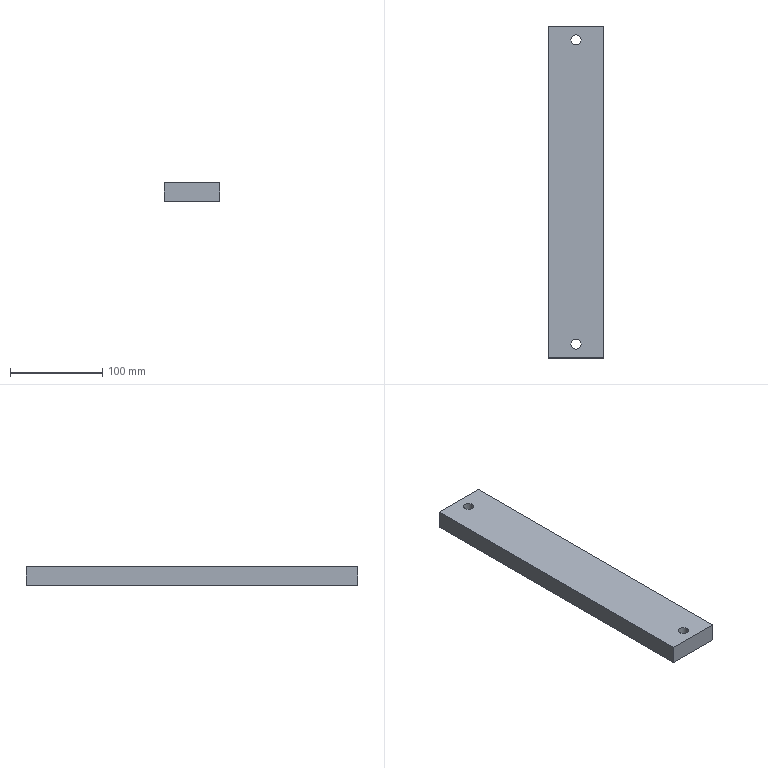Part | STEP file | 1 solid | 12 faces | box 60 x 360 x 20 mm | volume 425296 mm3 | plane 8 | cylinder 4 | commonest cylinder face diameters 11 x2 17 x2
STEP:
#1=CARTESIAN_POINT('',(0.,0.,0.));
#2=DIRECTION('',(0.,0.,1.));
#3=DIRECTION('',(1.,0.,0.));
#4=AXIS2_PLACEMENT_3D('',#1,#2,#3);
#5=CARTESIAN_POINT('',(1452.247,622.48,-145.381));
#6=VERTEX_POINT('',#5);
#7=CARTESIAN_POINT('',(1512.247,622.48,-145.381));
#8=VERTEX_POINT('',#7);
#9=CARTESIAN_POINT('',(1452.247,622.48,-145.381));
#10=DIRECTION('',(1.,0.,0.));
#11=VECTOR('',#10,1.);
#12=LINE('',#9,#11);
#13=CARTESIAN_POINT('',(1452.247,622.48,-165.381));
#14=DIRECTION('',(0.,-1.,0.));
#15=DIRECTION('',(0.,0.,1.));
#16=AXIS2_PLACEMENT_3D('',#13,#14,#15);
#17=PLANE('',#16);
#18=CARTESIAN_POINT('',(20.,0.));
#19=DIRECTION('',(0.,-1.));
#20=VECTOR('',#19,1.);
#21=LINE('',#18,#20);
#22=(GEOMETRIC_REPRESENTATION_CONTEXT(2)PARAMETRIC_REPRESENTATION_CONTEXT()REPRESENTATION_CONTEXT('',''));
#23=DEFINITIONAL_REPRESENTATION('',(#21),#22);
#24=PCURVE('',#17,#23);
#25=CARTESIAN_POINT('',(-340.,0.,-145.381));
#26=DIRECTION('',(0.,0.,-1.));
#27=DIRECTION('',(1.,0.,0.));
#28=AXIS2_PLACEMENT_3D('',#25,#26,#27);
#29=PLANE('',#28);
#30=CARTESIAN_POINT('',(1792.247,-622.48));
#31=DIRECTION('',(1.,0.));
#32=VECTOR('',#31,1.);
#33=LINE('',#30,#32);
#34=(GEOMETRIC_REPRESENTATION_CONTEXT(2)PARAMETRIC_REPRESENTATION_CONTEXT()REPRESENTATION_CONTEXT('',''));
#35=DEFINITIONAL_REPRESENTATION('',(#33),#34);
#36=PCURVE('',#29,#35);
#37=SURFACE_CURVE('',#12,(#24,#36),.PCURVE_S1.);
#38=EDGE_CURVE('',#6,#8,#37,.T.);
#39=ORIENTED_EDGE('',*,*,#38,.T.);
#40=CARTESIAN_POINT('',(1512.247,622.48,-165.381));
#41=VERTEX_POINT('',#40);
#42=CARTESIAN_POINT('',(1512.247,622.48,-165.381));
#43=DIRECTION('',(0.,0.,1.));
#44=VECTOR('',#43,1.);
#45=LINE('',#42,#44);
#46=CARTESIAN_POINT('',(0.,-60.));
#47=DIRECTION('',(1.,0.));
#48=VECTOR('',#47,1.);
#49=LINE('',#46,#48);
#50=(GEOMETRIC_REPRESENTATION_CONTEXT(2)PARAMETRIC_REPRESENTATION_CONTEXT()REPRESENTATION_CONTEXT('',''));
#51=DEFINITIONAL_REPRESENTATION('',(#49),#50);
#52=PCURVE('',#17,#51);
#53=CARTESIAN_POINT('',(1512.247,632.48,-165.381));
#54=DIRECTION('',(-1.,0.,0.));
#55=DIRECTION('',(0.,0.,-1.));
#56=AXIS2_PLACEMENT_3D('',#53,#54,#55);
#57=PLANE('',#56);
#58=CARTESIAN_POINT('',(0.,10.));
#59=DIRECTION('',(-1.,0.));
#60=VECTOR('',#59,1.);
#61=LINE('',#58,#60);
#62=(GEOMETRIC_REPRESENTATION_CONTEXT(2)PARAMETRIC_REPRESENTATION_CONTEXT()REPRESENTATION_CONTEXT('',''));
#63=DEFINITIONAL_REPRESENTATION('',(#61),#62);
#64=PCURVE('',#57,#63);
#65=SURFACE_CURVE('',#45,(#52,#64),.PCURVE_S1.);
#66=EDGE_CURVE('',#41,#8,#65,.T.);
#67=ORIENTED_EDGE('',*,*,#66,.F.);
#68=CARTESIAN_POINT('',(1452.247,622.48,-165.381));
#69=VERTEX_POINT('',#68);
#70=CARTESIAN_POINT('',(1452.247,622.48,-165.381));
#71=DIRECTION('',(1.,0.,0.));
#72=VECTOR('',#71,1.);
#73=LINE('',#70,#72);
#74=CARTESIAN_POINT('',(0.,0.));
#75=DIRECTION('',(0.,-1.));
#76=VECTOR('',#75,1.);
#77=LINE('',#74,#76);
#78=(GEOMETRIC_REPRESENTATION_CONTEXT(2)PARAMETRIC_REPRESENTATION_CONTEXT()REPRESENTATION_CONTEXT('',''));
#79=DEFINITIONAL_REPRESENTATION('',(#77),#78);
#80=PCURVE('',#17,#79);
#81=CARTESIAN_POINT('',(-340.,0.,-165.381));
#82=DIRECTION('',(0.,0.,-1.));
#83=DIRECTION('',(1.,0.,0.));
#84=AXIS2_PLACEMENT_3D('',#81,#82,#83);
#85=PLANE('',#84);
#86=CARTESIAN_POINT('',(1792.247,-622.48));
#87=DIRECTION('',(1.,0.));
#88=VECTOR('',#87,1.);
#89=LINE('',#86,#88);
#90=(GEOMETRIC_REPRESENTATION_CONTEXT(2)PARAMETRIC_REPRESENTATION_CONTEXT()REPRESENTATION_CONTEXT('',''));
#91=DEFINITIONAL_REPRESENTATION('',(#89),#90);
#92=PCURVE('',#85,#91);
#93=SURFACE_CURVE('',#73,(#80,#92),.PCURVE_S1.);
#94=EDGE_CURVE('',#69,#41,#93,.T.);
#95=ORIENTED_EDGE('',*,*,#94,.F.);
#96=CARTESIAN_POINT('',(1452.247,622.48,-165.381));
#97=DIRECTION('',(0.,0.,1.));
#98=VECTOR('',#97,1.);
#99=LINE('',#96,#98);
#100=CARTESIAN_POINT('',(0.,0.));
#101=DIRECTION('',(1.,0.));
#102=VECTOR('',#101,1.);
#103=LINE('',#100,#102);
#104=(GEOMETRIC_REPRESENTATION_CONTEXT(2)PARAMETRIC_REPRESENTATION_CONTEXT()REPRESENTATION_CONTEXT('',''));
#105=DEFINITIONAL_REPRESENTATION('',(#103),#104);
#106=PCURVE('',#17,#105);
#107=CARTESIAN_POINT('',(1452.247,252.48,-165.381));
#108=DIRECTION('',(1.,0.,0.));
#109=DIRECTION('',(0.,0.,1.));
#110=AXIS2_PLACEMENT_3D('',#107,#108,#109);
#111=PLANE('',#110);
#112=CARTESIAN_POINT('',(0.,-370.));
#113=DIRECTION('',(1.,0.));
#114=VECTOR('',#113,1.);
#115=LINE('',#112,#114);
#116=(GEOMETRIC_REPRESENTATION_CONTEXT(2)PARAMETRIC_REPRESENTATION_CONTEXT()REPRESENTATION_CONTEXT('',''));
#117=DEFINITIONAL_REPRESENTATION('',(#115),#116);
#118=PCURVE('',#111,#117);
#119=SURFACE_CURVE('',#99,(#106,#118),.PCURVE_S1.);
#120=EDGE_CURVE('',#69,#6,#119,.T.);
#121=ORIENTED_EDGE('',*,*,#120,.T.);
#122=EDGE_LOOP('',(#39,#67,#95,#121));
#123=FACE_BOUND('',#122,.T.);
#124=ADVANCED_FACE('',(#123),#17,.F.);
#125=CARTESIAN_POINT('',(1512.247,262.48,-145.381));
#126=VERTEX_POINT('',#125);
#127=CARTESIAN_POINT('',(1512.247,632.48,-145.381));
#128=DIRECTION('',(0.,-1.,0.));
#129=VECTOR('',#128,1.);
#130=LINE('',#127,#129);
#131=CARTESIAN_POINT('',(-20.,0.));
#132=DIRECTION('',(0.,1.));
#133=VECTOR('',#132,1.);
#134=LINE('',#131,#133);
#135=(GEOMETRIC_REPRESENTATION_CONTEXT(2)PARAMETRIC_REPRESENTATION_CONTEXT()REPRESENTATION_CONTEXT('',''));
#136=DEFINITIONAL_REPRESENTATION('',(#134),#135);
#137=PCURVE('',#57,#136);
#138=CARTESIAN_POINT('',(1852.247,-632.48));
#139=DIRECTION('',(0.,1.));
#140=VECTOR('',#139,1.);
#141=LINE('',#138,#140);
#142=(GEOMETRIC_REPRESENTATION_CONTEXT(2)PARAMETRIC_REPRESENTATION_CONTEXT()REPRESENTATION_CONTEXT('',''));
#143=DEFINITIONAL_REPRESENTATION('',(#141),#142);
#144=PCURVE('',#29,#143);
#145=SURFACE_CURVE('',#130,(#137,#144),.PCURVE_S1.);
#146=EDGE_CURVE('',#8,#126,#145,.T.);
#147=ORIENTED_EDGE('',*,*,#146,.T.);
#148=CARTESIAN_POINT('',(1512.247,262.48,-165.381));
#149=VERTEX_POINT('',#148);
#150=CARTESIAN_POINT('',(1512.247,262.48,-165.381));
#151=DIRECTION('',(0.,0.,1.));
#152=VECTOR('',#151,1.);
#153=LINE('',#150,#152);
#154=CARTESIAN_POINT('',(0.,370.));
#155=DIRECTION('',(-1.,0.));
#156=VECTOR('',#155,1.);
#157=LINE('',#154,#156);
#158=(GEOMETRIC_REPRESENTATION_CONTEXT(2)PARAMETRIC_REPRESENTATION_CONTEXT()REPRESENTATION_CONTEXT('',''));
#159=DEFINITIONAL_REPRESENTATION('',(#157),#158);
#160=PCURVE('',#57,#159);
#161=CARTESIAN_POINT('',(1512.247,262.48,-165.381));
#162=DIRECTION('',(0.,1.,0.));
#163=DIRECTION('',(1.,0.,0.));
#164=AXIS2_PLACEMENT_3D('',#161,#162,#163);
#165=PLANE('',#164);
#166=CARTESIAN_POINT('',(0.,0.));
#167=DIRECTION('',(0.,-1.));
#168=VECTOR('',#167,1.);
#169=LINE('',#166,#168);
#170=(GEOMETRIC_REPRESENTATION_CONTEXT(2)PARAMETRIC_REPRESENTATION_CONTEXT()REPRESENTATION_CONTEXT('',''));
#171=DEFINITIONAL_REPRESENTATION('',(#169),#170);
#172=PCURVE('',#165,#171);
#173=SURFACE_CURVE('',#153,(#160,#172),.PCURVE_S1.);
#174=EDGE_CURVE('',#149,#126,#173,.T.);
#175=ORIENTED_EDGE('',*,*,#174,.F.);
#176=CARTESIAN_POINT('',(1512.247,632.48,-165.381));
#177=DIRECTION('',(0.,-1.,0.));
#178=VECTOR('',#177,1.);
#179=LINE('',#176,#178);
#180=CARTESIAN_POINT('',(0.,0.));
#181=DIRECTION('',(0.,1.));
#182=VECTOR('',#181,1.);
#183=LINE('',#180,#182);
#184=(GEOMETRIC_REPRESENTATION_CONTEXT(2)PARAMETRIC_REPRESENTATION_CONTEXT()REPRESENTATION_CONTEXT('',''));
#185=DEFINITIONAL_REPRESENTATION('',(#183),#184);
#186=PCURVE('',#57,#185);
#187=CARTESIAN_POINT('',(1852.247,-632.48));
#188=DIRECTION('',(0.,1.));
#189=VECTOR('',#188,1.);
#190=LINE('',#187,#189);
#191=(GEOMETRIC_REPRESENTATION_CONTEXT(2)PARAMETRIC_REPRESENTATION_CONTEXT()REPRESENTATION_CONTEXT('',''));
#192=DEFINITIONAL_REPRESENTATION('',(#190),#191);
#193=PCURVE('',#85,#192);
#194=SURFACE_CURVE('',#179,(#186,#193),.PCURVE_S1.);
#195=EDGE_CURVE('',#41,#149,#194,.T.);
#196=ORIENTED_EDGE('',*,*,#195,.F.);
#197=ORIENTED_EDGE('',*,*,#66,.T.);
#198=EDGE_LOOP('',(#147,#175,#196,#197));
#199=FACE_BOUND('',#198,.T.);
#200=ADVANCED_FACE('',(#199),#57,.F.);
#201=CARTESIAN_POINT('',(1452.247,262.48,-145.381));
#202=VERTEX_POINT('',#201);
#203=CARTESIAN_POINT('',(1512.247,262.48,-145.381));
#204=DIRECTION('',(-1.,0.,0.));
#205=VECTOR('',#204,1.);
#206=LINE('',#203,#205);
#207=CARTESIAN_POINT('',(0.,-20.));
#208=DIRECTION('',(-1.,0.));
#209=VECTOR('',#208,1.);
#210=LINE('',#207,#209);
#211=(GEOMETRIC_REPRESENTATION_CONTEXT(2)PARAMETRIC_REPRESENTATION_CONTEXT()REPRESENTATION_CONTEXT('',''));
#212=DEFINITIONAL_REPRESENTATION('',(#210),#211);
#213=PCURVE('',#165,#212);
#214=CARTESIAN_POINT('',(1852.247,-262.48));
#215=DIRECTION('',(-1.,0.));
#216=VECTOR('',#215,1.);
#217=LINE('',#214,#216);
#218=(GEOMETRIC_REPRESENTATION_CONTEXT(2)PARAMETRIC_REPRESENTATION_CONTEXT()REPRESENTATION_CONTEXT('',''));
#219=DEFINITIONAL_REPRESENTATION('',(#217),#218);
#220=PCURVE('',#29,#219);
#221=SURFACE_CURVE('',#206,(#213,#220),.PCURVE_S1.);
#222=EDGE_CURVE('',#126,#202,#221,.T.);
#223=ORIENTED_EDGE('',*,*,#222,.T.);
#224=CARTESIAN_POINT('',(1452.247,262.48,-165.381));
#225=VERTEX_POINT('',#224);
#226=CARTESIAN_POINT('',(1452.247,262.48,-165.381));
#227=DIRECTION('',(0.,0.,1.));
#228=VECTOR('',#227,1.);
#229=LINE('',#226,#228);
#230=CARTESIAN_POINT('',(-60.,0.));
#231=DIRECTION('',(0.,-1.));
#232=VECTOR('',#231,1.);
#233=LINE('',#230,#232);
#234=(GEOMETRIC_REPRESENTATION_CONTEXT(2)PARAMETRIC_REPRESENTATION_CONTEXT()REPRESENTATION_CONTEXT('',''));
#235=DEFINITIONAL_REPRESENTATION('',(#233),#234);
#236=PCURVE('',#165,#235);
#237=CARTESIAN_POINT('',(0.,-10.));
#238=DIRECTION('',(1.,0.));
#239=VECTOR('',#238,1.);
#240=LINE('',#237,#239);
#241=(GEOMETRIC_REPRESENTATION_CONTEXT(2)PARAMETRIC_REPRESENTATION_CONTEXT()REPRESENTATION_CONTEXT('',''));
#242=DEFINITIONAL_REPRESENTATION('',(#240),#241);
#243=PCURVE('',#111,#242);
#244=SURFACE_CURVE('',#229,(#236,#243),.PCURVE_S1.);
#245=EDGE_CURVE('',#225,#202,#244,.T.);
#246=ORIENTED_EDGE('',*,*,#245,.F.);
#247=CARTESIAN_POINT('',(1512.247,262.48,-165.381));
#248=DIRECTION('',(-1.,0.,0.));
#249=VECTOR('',#248,1.);
#250=LINE('',#247,#249);
#251=CARTESIAN_POINT('',(0.,0.));
#252=DIRECTION('',(-1.,0.));
#253=VECTOR('',#252,1.);
#254=LINE('',#251,#253);
#255=(GEOMETRIC_REPRESENTATION_CONTEXT(2)PARAMETRIC_REPRESENTATION_CONTEXT()REPRESENTATION_CONTEXT('',''));
#256=DEFINITIONAL_REPRESENTATION('',(#254),#255);
#257=PCURVE('',#165,#256);
#258=CARTESIAN_POINT('',(1852.247,-262.48));
#259=DIRECTION('',(-1.,0.));
#260=VECTOR('',#259,1.);
#261=LINE('',#258,#260);
#262=(GEOMETRIC_REPRESENTATION_CONTEXT(2)PARAMETRIC_REPRESENTATION_CONTEXT()REPRESENTATION_CONTEXT('',''));
#263=DEFINITIONAL_REPRESENTATION('',(#261),#262);
#264=PCURVE('',#85,#263);
#265=SURFACE_CURVE('',#250,(#257,#264),.PCURVE_S1.);
#266=EDGE_CURVE('',#149,#225,#265,.T.);
#267=ORIENTED_EDGE('',*,*,#266,.F.);
#268=ORIENTED_EDGE('',*,*,#174,.T.);
#269=EDGE_LOOP('',(#223,#246,#267,#268));
#270=FACE_BOUND('',#269,.T.);
#271=ADVANCED_FACE('',(#270),#165,.F.);
#272=CARTESIAN_POINT('',(1452.247,252.48,-145.381));
#273=DIRECTION('',(0.,1.,0.));
#274=VECTOR('',#273,1.);
#275=LINE('',#272,#274);
#276=CARTESIAN_POINT('',(20.,0.));
#277=DIRECTION('',(0.,-1.));
#278=VECTOR('',#277,1.);
#279=LINE('',#276,#278);
#280=(GEOMETRIC_REPRESENTATION_CONTEXT(2)PARAMETRIC_REPRESENTATION_CONTEXT()REPRESENTATION_CONTEXT('',''));
#281=DEFINITIONAL_REPRESENTATION('',(#279),#280);
#282=PCURVE('',#111,#281);
#283=CARTESIAN_POINT('',(1792.247,-252.48));
#284=DIRECTION('',(0.,-1.));
#285=VECTOR('',#284,1.);
#286=LINE('',#283,#285);
#287=(GEOMETRIC_REPRESENTATION_CONTEXT(2)PARAMETRIC_REPRESENTATION_CONTEXT()REPRESENTATION_CONTEXT('',''));
#288=DEFINITIONAL_REPRESENTATION('',(#286),#287);
#289=PCURVE('',#29,#288);
#290=SURFACE_CURVE('',#275,(#282,#289),.PCURVE_S1.);
#291=EDGE_CURVE('',#202,#6,#290,.T.);
#292=ORIENTED_EDGE('',*,*,#291,.T.);
#293=ORIENTED_EDGE('',*,*,#120,.F.);
#294=CARTESIAN_POINT('',(1452.247,252.48,-165.381));
#295=DIRECTION('',(0.,1.,0.));
#296=VECTOR('',#295,1.);
#297=LINE('',#294,#296);
#298=CARTESIAN_POINT('',(0.,0.));
#299=DIRECTION('',(0.,-1.));
#300=VECTOR('',#299,1.);
#301=LINE('',#298,#300);
#302=(GEOMETRIC_REPRESENTATION_CONTEXT(2)PARAMETRIC_REPRESENTATION_CONTEXT()REPRESENTATION_CONTEXT('',''));
#303=DEFINITIONAL_REPRESENTATION('',(#301),#302);
#304=PCURVE('',#111,#303);
#305=CARTESIAN_POINT('',(1792.247,-252.48));
#306=DIRECTION('',(0.,-1.));
#307=VECTOR('',#306,1.);
#308=LINE('',#305,#307);
#309=(GEOMETRIC_REPRESENTATION_CONTEXT(2)PARAMETRIC_REPRESENTATION_CONTEXT()REPRESENTATION_CONTEXT('',''));
#310=DEFINITIONAL_REPRESENTATION('',(#308),#309);
#311=PCURVE('',#85,#310);
#312=SURFACE_CURVE('',#297,(#304,#311),.PCURVE_S1.);
#313=EDGE_CURVE('',#225,#69,#312,.T.);
#314=ORIENTED_EDGE('',*,*,#313,.F.);
#315=ORIENTED_EDGE('',*,*,#245,.T.);
#316=EDGE_LOOP('',(#292,#293,#314,#315));
#317=FACE_BOUND('',#316,.T.);
#318=ADVANCED_FACE('',(#317),#111,.F.);
#319=CARTESIAN_POINT('',(1473.747,277.48,-165.381));
#320=VERTEX_POINT('',#319);
#321=CARTESIAN_POINT('',(1482.247,277.48,-165.381));
#322=DIRECTION('',(0.,0.,1.));
#323=DIRECTION('',(-1.,0.,0.));
#324=AXIS2_PLACEMENT_3D('',#321,#322,#323);
#325=CIRCLE('',#324,8.5);
#326=CARTESIAN_POINT('',(1813.747,-277.48));
#327=CARTESIAN_POINT('',(1813.747,-262.758));
#328=CARTESIAN_POINT('',(1826.497,-270.119));
#329=CARTESIAN_POINT('',(1839.247,-277.48));
#330=CARTESIAN_POINT('',(1826.497,-284.842));
#331=CARTESIAN_POINT('',(1813.747,-292.203));
#332=CARTESIAN_POINT('',(1813.747,-277.48));
#333=(BOUNDED_CURVE()B_SPLINE_CURVE(2,(#326,#327,#328,#329,#330,#331,#332),.UNSPECIFIED.,.T.,.F.)B_SPLINE_CURVE_WITH_KNOTS((1,2,2,2,2,1),(-2.094,0.,2.094,4.189,6.283,8.378),.UNSPECIFIED.)CURVE()GEOMETRIC_REPRESENTATION_ITEM()RATIONAL_B_SPLINE_CURVE((1.,0.5,1.,0.5,1.,0.5,1.))REPRESENTATION_ITEM(''));
#334=(GEOMETRIC_REPRESENTATION_CONTEXT(2)PARAMETRIC_REPRESENTATION_CONTEXT()REPRESENTATION_CONTEXT('',''));
#335=DEFINITIONAL_REPRESENTATION('',(#333),#334);
#336=PCURVE('',#85,#335);
#337=CARTESIAN_POINT('',(1482.247,277.48,-165.381));
#338=DIRECTION('',(0.,0.,1.));
#339=DIRECTION('',(-1.,0.,0.));
#340=AXIS2_PLACEMENT_3D('',#337,#338,#339);
#341=CYLINDRICAL_SURFACE('',#340,8.5);
#342=CARTESIAN_POINT('',(0.,0.));
#343=DIRECTION('',(1.,0.));
#344=VECTOR('',#343,1.);
#345=LINE('',#342,#344);
#346=(GEOMETRIC_REPRESENTATION_CONTEXT(2)PARAMETRIC_REPRESENTATION_CONTEXT()REPRESENTATION_CONTEXT('',''));
#347=DEFINITIONAL_REPRESENTATION('',(#345),#346);
#348=PCURVE('',#341,#347);
#349=SURFACE_CURVE('',#325,(#336,#348),.PCURVE_S1.);
#350=EDGE_CURVE('',#320,#320,#349,.T.);
#351=ORIENTED_EDGE('',*,*,#350,.T.);
#352=EDGE_LOOP('',(#351));
#353=FACE_BOUND('',#352,.T.);
#354=CARTESIAN_POINT('',(1473.747,607.48,-165.381));
#355=VERTEX_POINT('',#354);
#356=CARTESIAN_POINT('',(1482.247,607.48,-165.381));
#357=DIRECTION('',(0.,0.,1.));
#358=DIRECTION('',(-1.,0.,0.));
#359=AXIS2_PLACEMENT_3D('',#356,#357,#358);
#360=CIRCLE('',#359,8.5);
#361=CARTESIAN_POINT('',(1813.747,-607.48));
#362=CARTESIAN_POINT('',(1813.747,-592.758));
#363=CARTESIAN_POINT('',(1826.497,-600.119));
#364=CARTESIAN_POINT('',(1839.247,-607.48));
#365=CARTESIAN_POINT('',(1826.497,-614.842));
#366=CARTESIAN_POINT('',(1813.747,-622.203));
#367=CARTESIAN_POINT('',(1813.747,-607.48));
#368=(BOUNDED_CURVE()B_SPLINE_CURVE(2,(#361,#362,#363,#364,#365,#366,#367),.UNSPECIFIED.,.T.,.F.)B_SPLINE_CURVE_WITH_KNOTS((1,2,2,2,2,1),(-2.094,0.,2.094,4.189,6.283,8.378),.UNSPECIFIED.)CURVE()GEOMETRIC_REPRESENTATION_ITEM()RATIONAL_B_SPLINE_CURVE((1.,0.5,1.,0.5,1.,0.5,1.))REPRESENTATION_ITEM(''));
#369=(GEOMETRIC_REPRESENTATION_CONTEXT(2)PARAMETRIC_REPRESENTATION_CONTEXT()REPRESENTATION_CONTEXT('',''));
#370=DEFINITIONAL_REPRESENTATION('',(#368),#369);
#371=PCURVE('',#85,#370);
#372=CARTESIAN_POINT('',(1482.247,607.48,-165.381));
#373=DIRECTION('',(0.,0.,1.));
#374=DIRECTION('',(-1.,0.,0.));
#375=AXIS2_PLACEMENT_3D('',#372,#373,#374);
#376=CYLINDRICAL_SURFACE('',#375,8.5);
#377=CARTESIAN_POINT('',(0.,0.));
#378=DIRECTION('',(1.,0.));
#379=VECTOR('',#378,1.);
#380=LINE('',#377,#379);
#381=(GEOMETRIC_REPRESENTATION_CONTEXT(2)PARAMETRIC_REPRESENTATION_CONTEXT()REPRESENTATION_CONTEXT('',''));
#382=DEFINITIONAL_REPRESENTATION('',(#380),#381);
#383=PCURVE('',#376,#382);
#384=SURFACE_CURVE('',#360,(#371,#383),.PCURVE_S1.);
#385=EDGE_CURVE('',#355,#355,#384,.T.);
#386=ORIENTED_EDGE('',*,*,#385,.T.);
#387=EDGE_LOOP('',(#386));
#388=FACE_BOUND('',#387,.T.);
#389=ORIENTED_EDGE('',*,*,#94,.T.);
#390=ORIENTED_EDGE('',*,*,#195,.T.);
#391=ORIENTED_EDGE('',*,*,#266,.T.);
#392=ORIENTED_EDGE('',*,*,#313,.T.);
#393=EDGE_LOOP('',(#389,#390,#391,#392));
#394=FACE_BOUND('',#393,.T.);
#395=ADVANCED_FACE('',(#353,#388,#394),#85,.T.);
#396=CARTESIAN_POINT('',(1476.747,277.48,-145.381));
#397=VERTEX_POINT('',#396);
#398=CARTESIAN_POINT('',(1482.247,277.48,-145.381));
#399=DIRECTION('',(0.,0.,-1.));
#400=DIRECTION('',(-1.,0.,0.));
#401=AXIS2_PLACEMENT_3D('',#398,#399,#400);
#402=CIRCLE('',#401,5.5);
#403=CARTESIAN_POINT('',(1822.247,-277.48));
#404=DIRECTION('',(-1.,0.));
#405=AXIS2_PLACEMENT_2D('',#403,#404);
#406=CIRCLE('',#405,5.5);
#407=(GEOMETRIC_REPRESENTATION_CONTEXT(2)PARAMETRIC_REPRESENTATION_CONTEXT()REPRESENTATION_CONTEXT('',''));
#408=DEFINITIONAL_REPRESENTATION('',(#406),#407);
#409=PCURVE('',#29,#408);
#410=CARTESIAN_POINT('',(1482.247,277.48,-40.538));
#411=DIRECTION('',(0.,0.,1.));
#412=DIRECTION('',(-1.,0.,0.));
#413=AXIS2_PLACEMENT_3D('',#410,#411,#412);
#414=CYLINDRICAL_SURFACE('',#413,5.5);
#415=CARTESIAN_POINT('',(6.283,-104.843));
#416=DIRECTION('',(-1.,0.));
#417=VECTOR('',#416,1.);
#418=LINE('',#415,#417);
#419=(GEOMETRIC_REPRESENTATION_CONTEXT(2)PARAMETRIC_REPRESENTATION_CONTEXT()REPRESENTATION_CONTEXT('',''));
#420=DEFINITIONAL_REPRESENTATION('',(#418),#419);
#421=PCURVE('',#414,#420);
#422=SURFACE_CURVE('',#402,(#409,#421),.PCURVE_S1.);
#423=EDGE_CURVE('',#397,#397,#422,.T.);
#424=ORIENTED_EDGE('',*,*,#423,.T.);
#425=EDGE_LOOP('',(#424));
#426=FACE_BOUND('',#425,.T.);
#427=CARTESIAN_POINT('',(1476.747,607.48,-145.381));
#428=VERTEX_POINT('',#427);
#429=CARTESIAN_POINT('',(1482.247,607.48,-145.381));
#430=DIRECTION('',(0.,0.,-1.));
#431=DIRECTION('',(-1.,0.,0.));
#432=AXIS2_PLACEMENT_3D('',#429,#430,#431);
#433=CIRCLE('',#432,5.5);
#434=CARTESIAN_POINT('',(1822.247,-607.48));
#435=DIRECTION('',(-1.,0.));
#436=AXIS2_PLACEMENT_2D('',#434,#435);
#437=CIRCLE('',#436,5.5);
#438=(GEOMETRIC_REPRESENTATION_CONTEXT(2)PARAMETRIC_REPRESENTATION_CONTEXT()REPRESENTATION_CONTEXT('',''));
#439=DEFINITIONAL_REPRESENTATION('',(#437),#438);
#440=PCURVE('',#29,#439);
#441=CARTESIAN_POINT('',(1482.247,607.48,-40.538));
#442=DIRECTION('',(0.,0.,1.));
#443=DIRECTION('',(-1.,0.,0.));
#444=AXIS2_PLACEMENT_3D('',#441,#442,#443);
#445=CYLINDRICAL_SURFACE('',#444,5.5);
#446=CARTESIAN_POINT('',(6.283,-104.843));
#447=DIRECTION('',(-1.,0.));
#448=VECTOR('',#447,1.);
#449=LINE('',#446,#448);
#450=(GEOMETRIC_REPRESENTATION_CONTEXT(2)PARAMETRIC_REPRESENTATION_CONTEXT()REPRESENTATION_CONTEXT('',''));
#451=DEFINITIONAL_REPRESENTATION('',(#449),#450);
#452=PCURVE('',#445,#451);
#453=SURFACE_CURVE('',#433,(#440,#452),.PCURVE_S1.);
#454=EDGE_CURVE('',#428,#428,#453,.T.);
#455=ORIENTED_EDGE('',*,*,#454,.T.);
#456=EDGE_LOOP('',(#455));
#457=FACE_BOUND('',#456,.T.);
#458=ORIENTED_EDGE('',*,*,#38,.F.);
#459=ORIENTED_EDGE('',*,*,#291,.F.);
#460=ORIENTED_EDGE('',*,*,#222,.F.);
#461=ORIENTED_EDGE('',*,*,#146,.F.);
#462=EDGE_LOOP('',(#458,#459,#460,#461));
#463=FACE_BOUND('',#462,.T.);
#464=ADVANCED_FACE('',(#426,#457,#463),#29,.F.);
#465=CARTESIAN_POINT('',(1476.747,607.48,-154.381));
#466=VERTEX_POINT('',#465);
#467=CARTESIAN_POINT('',(1487.747,607.48,-154.381));
#468=VERTEX_POINT('',#467);
#469=CARTESIAN_POINT('',(1482.247,607.48,-154.381));
#470=DIRECTION('',(0.,0.,-1.));
#471=DIRECTION('',(1.,0.,0.));
#472=AXIS2_PLACEMENT_3D('',#469,#470,#471);
#473=CIRCLE('',#472,5.5);
#474=CARTESIAN_POINT('',(9.425,-113.843));
#475=DIRECTION('',(-1.,0.));
#476=VECTOR('',#475,1.);
#477=LINE('',#474,#476);
#478=(GEOMETRIC_REPRESENTATION_CONTEXT(2)PARAMETRIC_REPRESENTATION_CONTEXT()REPRESENTATION_CONTEXT('',''));
#479=DEFINITIONAL_REPRESENTATION('',(#477),#478);
#480=PCURVE('',#445,#479);
#481=CARTESIAN_POINT('',(1482.247,607.48,-154.381));
#482=DIRECTION('',(0.,0.,1.));
#483=DIRECTION('',(-1.,0.,0.));
#484=AXIS2_PLACEMENT_3D('',#481,#482,#483);
#485=PLANE('',#484);
#486=CARTESIAN_POINT('',(-5.5,0.));
#487=CARTESIAN_POINT('',(-5.5,9.526));
#488=CARTESIAN_POINT('',(2.75,4.763));
#489=CARTESIAN_POINT('',(11.,0.));
#490=CARTESIAN_POINT('',(2.75,-4.763));
#491=CARTESIAN_POINT('',(-5.5,-9.526));
#492=CARTESIAN_POINT('',(-5.5,0.));
#493=(BOUNDED_CURVE()B_SPLINE_CURVE(2,(#486,#487,#488,#489,#490,#491,#492),.UNSPECIFIED.,.T.,.F.)B_SPLINE_CURVE_WITH_KNOTS((1,2,2,2,2,1),(-2.094,0.,2.094,4.189,6.283,8.378),.UNSPECIFIED.)CURVE()GEOMETRIC_REPRESENTATION_ITEM()RATIONAL_B_SPLINE_CURVE((1.,0.5,1.,0.5,1.,0.5,1.))REPRESENTATION_ITEM(''));
#494=(GEOMETRIC_REPRESENTATION_CONTEXT(2)PARAMETRIC_REPRESENTATION_CONTEXT()REPRESENTATION_CONTEXT('',''));
#495=DEFINITIONAL_REPRESENTATION('',(#493),#494);
#496=PCURVE('',#485,#495);
#497=SURFACE_CURVE('',#473,(#480,#496),.PCURVE_S1.);
#498=EDGE_CURVE('',#466,#468,#497,.T.);
#499=ORIENTED_EDGE('',*,*,#498,.F.);
#500=CARTESIAN_POINT('',(1476.747,607.48,-154.381));
#501=CARTESIAN_POINT('',(1476.747,607.48,-145.381));
#502=B_SPLINE_CURVE_WITH_KNOTS('',1,(#500,#501),.UNSPECIFIED.,.F.,.F.,(2,2),(-113.843,-104.843),.PIECEWISE_BEZIER_KNOTS.);
#503=CARTESIAN_POINT('',(6.283,0.));
#504=DIRECTION('',(0.,1.));
#505=VECTOR('',#504,1.);
#506=LINE('',#503,#505);
#507=(GEOMETRIC_REPRESENTATION_CONTEXT(2)PARAMETRIC_REPRESENTATION_CONTEXT()REPRESENTATION_CONTEXT('',''));
#508=DEFINITIONAL_REPRESENTATION('',(#506),#507);
#509=PCURVE('',#445,#508);
#510=CARTESIAN_POINT('',(0.,0.));
#511=DIRECTION('',(0.,1.));
#512=VECTOR('',#511,1.);
#513=LINE('',#510,#512);
#514=(GEOMETRIC_REPRESENTATION_CONTEXT(2)PARAMETRIC_REPRESENTATION_CONTEXT()REPRESENTATION_CONTEXT('',''));
#515=DEFINITIONAL_REPRESENTATION('',(#513),#514);
#516=PCURVE('',#445,#515);
#517=SEAM_CURVE('',#502,(#509,#516),.PCURVE_S1.);
#518=EDGE_CURVE('',#466,#428,#517,.T.);
#519=ORIENTED_EDGE('',*,*,#518,.T.);
#520=ORIENTED_EDGE('',*,*,#454,.T.);
#521=ORIENTED_EDGE('',*,*,#518,.F.);
#522=CARTESIAN_POINT('',(1482.247,607.48,-154.381));
#523=DIRECTION('',(0.,0.,-1.));
#524=DIRECTION('',(1.,0.,0.));
#525=AXIS2_PLACEMENT_3D('',#522,#523,#524);
#526=CIRCLE('',#525,5.5);
#527=CARTESIAN_POINT('',(3.142,-113.843));
#528=DIRECTION('',(-1.,0.));
#529=VECTOR('',#528,1.);
#530=LINE('',#527,#529);
#531=(GEOMETRIC_REPRESENTATION_CONTEXT(2)PARAMETRIC_REPRESENTATION_CONTEXT()REPRESENTATION_CONTEXT('',''));
#532=DEFINITIONAL_REPRESENTATION('',(#530),#531);
#533=PCURVE('',#445,#532);
#534=CARTESIAN_POINT('',(-5.5,0.));
#535=CARTESIAN_POINT('',(-5.5,9.526));
#536=CARTESIAN_POINT('',(2.75,4.763));
#537=CARTESIAN_POINT('',(11.,0.));
#538=CARTESIAN_POINT('',(2.75,-4.763));
#539=CARTESIAN_POINT('',(-5.5,-9.526));
#540=CARTESIAN_POINT('',(-5.5,0.));
#541=(BOUNDED_CURVE()B_SPLINE_CURVE(2,(#534,#535,#536,#537,#538,#539,#540),.UNSPECIFIED.,.T.,.F.)B_SPLINE_CURVE_WITH_KNOTS((1,2,2,2,2,1),(-2.094,0.,2.094,4.189,6.283,8.378),.UNSPECIFIED.)CURVE()GEOMETRIC_REPRESENTATION_ITEM()RATIONAL_B_SPLINE_CURVE((1.,0.5,1.,0.5,1.,0.5,1.))REPRESENTATION_ITEM(''));
#542=(GEOMETRIC_REPRESENTATION_CONTEXT(2)PARAMETRIC_REPRESENTATION_CONTEXT()REPRESENTATION_CONTEXT('',''));
#543=DEFINITIONAL_REPRESENTATION('',(#541),#542);
#544=PCURVE('',#485,#543);
#545=SURFACE_CURVE('',#526,(#533,#544),.PCURVE_S1.);
#546=EDGE_CURVE('',#468,#466,#545,.T.);
#547=ORIENTED_EDGE('',*,*,#546,.F.);
#548=EDGE_LOOP('',(#499,#519,#520,#521,#547));
#549=FACE_BOUND('',#548,.F.);
#550=ADVANCED_FACE('',(#549),#445,.F.);
#551=ORIENTED_EDGE('',*,*,#546,.F.);
#552=ORIENTED_EDGE('',*,*,#498,.F.);
#553=EDGE_LOOP('',(#551,#552));
#554=FACE_BOUND('',#553,.T.);
#555=CARTESIAN_POINT('',(1490.747,607.48,-154.381));
#556=VERTEX_POINT('',#555);
#557=CARTESIAN_POINT('',(1473.747,607.48,-154.381));
#558=VERTEX_POINT('',#557);
#559=CARTESIAN_POINT('',(1482.247,607.48,-154.381));
#560=DIRECTION('',(0.,0.,-1.));
#561=DIRECTION('',(1.,0.,0.));
#562=AXIS2_PLACEMENT_3D('',#559,#560,#561);
#563=CIRCLE('',#562,8.5);
#564=CARTESIAN_POINT('',(-8.5,0.));
#565=CARTESIAN_POINT('',(-8.5,14.722));
#566=CARTESIAN_POINT('',(4.25,7.361));
#567=CARTESIAN_POINT('',(17.,0.));
#568=CARTESIAN_POINT('',(4.25,-7.361));
#569=CARTESIAN_POINT('',(-8.5,-14.722));
#570=CARTESIAN_POINT('',(-8.5,0.));
#571=(BOUNDED_CURVE()B_SPLINE_CURVE(2,(#564,#565,#566,#567,#568,#569,#570),.UNSPECIFIED.,.T.,.F.)B_SPLINE_CURVE_WITH_KNOTS((1,2,2,2,2,1),(-2.094,0.,2.094,4.189,6.283,8.378),.UNSPECIFIED.)CURVE()GEOMETRIC_REPRESENTATION_ITEM()RATIONAL_B_SPLINE_CURVE((1.,0.5,1.,0.5,1.,0.5,1.))REPRESENTATION_ITEM(''));
#572=(GEOMETRIC_REPRESENTATION_CONTEXT(2)PARAMETRIC_REPRESENTATION_CONTEXT()REPRESENTATION_CONTEXT('',''));
#573=DEFINITIONAL_REPRESENTATION('',(#571),#572);
#574=PCURVE('',#485,#573);
#575=CARTESIAN_POINT('',(3.142,11.));
#576=DIRECTION('',(-1.,0.));
#577=VECTOR('',#576,1.);
#578=LINE('',#575,#577);
#579=(GEOMETRIC_REPRESENTATION_CONTEXT(2)PARAMETRIC_REPRESENTATION_CONTEXT()REPRESENTATION_CONTEXT('',''));
#580=DEFINITIONAL_REPRESENTATION('',(#578),#579);
#581=PCURVE('',#376,#580);
#582=SURFACE_CURVE('',#563,(#574,#581),.PCURVE_S1.);
#583=EDGE_CURVE('',#556,#558,#582,.T.);
#584=ORIENTED_EDGE('',*,*,#583,.T.);
#585=CARTESIAN_POINT('',(1482.247,607.48,-154.381));
#586=DIRECTION('',(0.,0.,-1.));
#587=DIRECTION('',(1.,0.,0.));
#588=AXIS2_PLACEMENT_3D('',#585,#586,#587);
#589=CIRCLE('',#588,8.5);
#590=CARTESIAN_POINT('',(-8.5,0.));
#591=CARTESIAN_POINT('',(-8.5,14.722));
#592=CARTESIAN_POINT('',(4.25,7.361));
#593=CARTESIAN_POINT('',(17.,0.));
#594=CARTESIAN_POINT('',(4.25,-7.361));
#595=CARTESIAN_POINT('',(-8.5,-14.722));
#596=CARTESIAN_POINT('',(-8.5,0.));
#597=(BOUNDED_CURVE()B_SPLINE_CURVE(2,(#590,#591,#592,#593,#594,#595,#596),.UNSPECIFIED.,.T.,.F.)B_SPLINE_CURVE_WITH_KNOTS((1,2,2,2,2,1),(-2.094,0.,2.094,4.189,6.283,8.378),.UNSPECIFIED.)CURVE()GEOMETRIC_REPRESENTATION_ITEM()RATIONAL_B_SPLINE_CURVE((1.,0.5,1.,0.5,1.,0.5,1.))REPRESENTATION_ITEM(''));
#598=(GEOMETRIC_REPRESENTATION_CONTEXT(2)PARAMETRIC_REPRESENTATION_CONTEXT()REPRESENTATION_CONTEXT('',''));
#599=DEFINITIONAL_REPRESENTATION('',(#597),#598);
#600=PCURVE('',#485,#599);
#601=CARTESIAN_POINT('',(9.425,11.));
#602=DIRECTION('',(-1.,0.));
#603=VECTOR('',#602,1.);
#604=LINE('',#601,#603);
#605=(GEOMETRIC_REPRESENTATION_CONTEXT(2)PARAMETRIC_REPRESENTATION_CONTEXT()REPRESENTATION_CONTEXT('',''));
#606=DEFINITIONAL_REPRESENTATION('',(#604),#605);
#607=PCURVE('',#376,#606);
#608=SURFACE_CURVE('',#589,(#600,#607),.PCURVE_S1.);
#609=EDGE_CURVE('',#558,#556,#608,.T.);
#610=ORIENTED_EDGE('',*,*,#609,.T.);
#611=EDGE_LOOP('',(#584,#610));
#612=FACE_BOUND('',#611,.T.);
#613=ADVANCED_FACE('',(#554,#612),#485,.F.);
#614=ORIENTED_EDGE('',*,*,#583,.T.);
#615=CARTESIAN_POINT('',(1473.747,607.48,-165.381));
#616=CARTESIAN_POINT('',(1473.747,607.48,-154.381));
#617=B_SPLINE_CURVE_WITH_KNOTS('',1,(#615,#616),.UNSPECIFIED.,.F.,.F.,(2,2),(0.,11.),.PIECEWISE_BEZIER_KNOTS.);
#618=CARTESIAN_POINT('',(0.,0.));
#619=DIRECTION('',(0.,1.));
#620=VECTOR('',#619,1.);
#621=LINE('',#618,#620);
#622=(GEOMETRIC_REPRESENTATION_CONTEXT(2)PARAMETRIC_REPRESENTATION_CONTEXT()REPRESENTATION_CONTEXT('',''));
#623=DEFINITIONAL_REPRESENTATION('',(#621),#622);
#624=PCURVE('',#376,#623);
#625=CARTESIAN_POINT('',(6.283,0.));
#626=DIRECTION('',(0.,1.));
#627=VECTOR('',#626,1.);
#628=LINE('',#625,#627);
#629=(GEOMETRIC_REPRESENTATION_CONTEXT(2)PARAMETRIC_REPRESENTATION_CONTEXT()REPRESENTATION_CONTEXT('',''));
#630=DEFINITIONAL_REPRESENTATION('',(#628),#629);
#631=PCURVE('',#376,#630);
#632=SEAM_CURVE('',#617,(#624,#631),.PCURVE_S1.);
#633=EDGE_CURVE('',#355,#558,#632,.T.);
#634=ORIENTED_EDGE('',*,*,#633,.F.);
#635=ORIENTED_EDGE('',*,*,#385,.T.);
#636=ORIENTED_EDGE('',*,*,#633,.T.);
#637=ORIENTED_EDGE('',*,*,#609,.T.);
#638=EDGE_LOOP('',(#614,#634,#635,#636,#637));
#639=FACE_BOUND('',#638,.F.);
#640=ADVANCED_FACE('',(#639),#376,.F.);
#641=CARTESIAN_POINT('',(1476.747,277.48,-154.381));
#642=VERTEX_POINT('',#641);
#643=CARTESIAN_POINT('',(1487.747,277.48,-154.381));
#644=VERTEX_POINT('',#643);
#645=CARTESIAN_POINT('',(1482.247,277.48,-154.381));
#646=DIRECTION('',(0.,0.,-1.));
#647=DIRECTION('',(1.,0.,0.));
#648=AXIS2_PLACEMENT_3D('',#645,#646,#647);
#649=CIRCLE('',#648,5.5);
#650=CARTESIAN_POINT('',(9.425,-113.843));
#651=DIRECTION('',(-1.,0.));
#652=VECTOR('',#651,1.);
#653=LINE('',#650,#652);
#654=(GEOMETRIC_REPRESENTATION_CONTEXT(2)PARAMETRIC_REPRESENTATION_CONTEXT()REPRESENTATION_CONTEXT('',''));
#655=DEFINITIONAL_REPRESENTATION('',(#653),#654);
#656=PCURVE('',#414,#655);
#657=CARTESIAN_POINT('',(1482.247,277.48,-154.381));
#658=DIRECTION('',(0.,0.,1.));
#659=DIRECTION('',(-1.,0.,0.));
#660=AXIS2_PLACEMENT_3D('',#657,#658,#659);
#661=PLANE('',#660);
#662=CARTESIAN_POINT('',(-5.5,0.));
#663=CARTESIAN_POINT('',(-5.5,9.526));
#664=CARTESIAN_POINT('',(2.75,4.763));
#665=CARTESIAN_POINT('',(11.,0.));
#666=CARTESIAN_POINT('',(2.75,-4.763));
#667=CARTESIAN_POINT('',(-5.5,-9.526));
#668=CARTESIAN_POINT('',(-5.5,0.));
#669=(BOUNDED_CURVE()B_SPLINE_CURVE(2,(#662,#663,#664,#665,#666,#667,#668),.UNSPECIFIED.,.T.,.F.)B_SPLINE_CURVE_WITH_KNOTS((1,2,2,2,2,1),(-2.094,0.,2.094,4.189,6.283,8.378),.UNSPECIFIED.)CURVE()GEOMETRIC_REPRESENTATION_ITEM()RATIONAL_B_SPLINE_CURVE((1.,0.5,1.,0.5,1.,0.5,1.))REPRESENTATION_ITEM(''));
#670=(GEOMETRIC_REPRESENTATION_CONTEXT(2)PARAMETRIC_REPRESENTATION_CONTEXT()REPRESENTATION_CONTEXT('',''));
#671=DEFINITIONAL_REPRESENTATION('',(#669),#670);
#672=PCURVE('',#661,#671);
#673=SURFACE_CURVE('',#649,(#656,#672),.PCURVE_S1.);
#674=EDGE_CURVE('',#642,#644,#673,.T.);
#675=ORIENTED_EDGE('',*,*,#674,.F.);
#676=CARTESIAN_POINT('',(1476.747,277.48,-154.381));
#677=CARTESIAN_POINT('',(1476.747,277.48,-145.381));
#678=B_SPLINE_CURVE_WITH_KNOTS('',1,(#676,#677),.UNSPECIFIED.,.F.,.F.,(2,2),(-113.843,-104.843),.PIECEWISE_BEZIER_KNOTS.);
#679=CARTESIAN_POINT('',(6.283,0.));
#680=DIRECTION('',(0.,1.));
#681=VECTOR('',#680,1.);
#682=LINE('',#679,#681);
#683=(GEOMETRIC_REPRESENTATION_CONTEXT(2)PARAMETRIC_REPRESENTATION_CONTEXT()REPRESENTATION_CONTEXT('',''));
#684=DEFINITIONAL_REPRESENTATION('',(#682),#683);
#685=PCURVE('',#414,#684);
#686=CARTESIAN_POINT('',(0.,0.));
#687=DIRECTION('',(0.,1.));
#688=VECTOR('',#687,1.);
#689=LINE('',#686,#688);
#690=(GEOMETRIC_REPRESENTATION_CONTEXT(2)PARAMETRIC_REPRESENTATION_CONTEXT()REPRESENTATION_CONTEXT('',''));
#691=DEFINITIONAL_REPRESENTATION('',(#689),#690);
#692=PCURVE('',#414,#691);
#693=SEAM_CURVE('',#678,(#685,#692),.PCURVE_S1.);
#694=EDGE_CURVE('',#642,#397,#693,.T.);
#695=ORIENTED_EDGE('',*,*,#694,.T.);
#696=ORIENTED_EDGE('',*,*,#423,.T.);
#697=ORIENTED_EDGE('',*,*,#694,.F.);
#698=CARTESIAN_POINT('',(1482.247,277.48,-154.381));
#699=DIRECTION('',(0.,0.,-1.));
#700=DIRECTION('',(1.,0.,0.));
#701=AXIS2_PLACEMENT_3D('',#698,#699,#700);
#702=CIRCLE('',#701,5.5);
#703=CARTESIAN_POINT('',(3.142,-113.843));
#704=DIRECTION('',(-1.,0.));
#705=VECTOR('',#704,1.);
#706=LINE('',#703,#705);
#707=(GEOMETRIC_REPRESENTATION_CONTEXT(2)PARAMETRIC_REPRESENTATION_CONTEXT()REPRESENTATION_CONTEXT('',''));
#708=DEFINITIONAL_REPRESENTATION('',(#706),#707);
#709=PCURVE('',#414,#708);
#710=CARTESIAN_POINT('',(-5.5,0.));
#711=CARTESIAN_POINT('',(-5.5,9.526));
#712=CARTESIAN_POINT('',(2.75,4.763));
#713=CARTESIAN_POINT('',(11.,0.));
#714=CARTESIAN_POINT('',(2.75,-4.763));
#715=CARTESIAN_POINT('',(-5.5,-9.526));
#716=CARTESIAN_POINT('',(-5.5,0.));
#717=(BOUNDED_CURVE()B_SPLINE_CURVE(2,(#710,#711,#712,#713,#714,#715,#716),.UNSPECIFIED.,.T.,.F.)B_SPLINE_CURVE_WITH_KNOTS((1,2,2,2,2,1),(-2.094,0.,2.094,4.189,6.283,8.378),.UNSPECIFIED.)CURVE()GEOMETRIC_REPRESENTATION_ITEM()RATIONAL_B_SPLINE_CURVE((1.,0.5,1.,0.5,1.,0.5,1.))REPRESENTATION_ITEM(''));
#718=(GEOMETRIC_REPRESENTATION_CONTEXT(2)PARAMETRIC_REPRESENTATION_CONTEXT()REPRESENTATION_CONTEXT('',''));
#719=DEFINITIONAL_REPRESENTATION('',(#717),#718);
#720=PCURVE('',#661,#719);
#721=SURFACE_CURVE('',#702,(#709,#720),.PCURVE_S1.);
#722=EDGE_CURVE('',#644,#642,#721,.T.);
#723=ORIENTED_EDGE('',*,*,#722,.F.);
#724=EDGE_LOOP('',(#675,#695,#696,#697,#723));
#725=FACE_BOUND('',#724,.F.);
#726=ADVANCED_FACE('',(#725),#414,.F.);
#727=ORIENTED_EDGE('',*,*,#722,.F.);
#728=ORIENTED_EDGE('',*,*,#674,.F.);
#729=EDGE_LOOP('',(#727,#728));
#730=FACE_BOUND('',#729,.T.);
#731=CARTESIAN_POINT('',(1490.747,277.48,-154.381));
#732=VERTEX_POINT('',#731);
#733=CARTESIAN_POINT('',(1473.747,277.48,-154.381));
#734=VERTEX_POINT('',#733);
#735=CARTESIAN_POINT('',(1482.247,277.48,-154.381));
#736=DIRECTION('',(0.,0.,-1.));
#737=DIRECTION('',(1.,0.,0.));
#738=AXIS2_PLACEMENT_3D('',#735,#736,#737);
#739=CIRCLE('',#738,8.5);
#740=CARTESIAN_POINT('',(-8.5,0.));
#741=CARTESIAN_POINT('',(-8.5,14.722));
#742=CARTESIAN_POINT('',(4.25,7.361));
#743=CARTESIAN_POINT('',(17.,0.));
#744=CARTESIAN_POINT('',(4.25,-7.361));
#745=CARTESIAN_POINT('',(-8.5,-14.722));
#746=CARTESIAN_POINT('',(-8.5,0.));
#747=(BOUNDED_CURVE()B_SPLINE_CURVE(2,(#740,#741,#742,#743,#744,#745,#746),.UNSPECIFIED.,.T.,.F.)B_SPLINE_CURVE_WITH_KNOTS((1,2,2,2,2,1),(-2.094,0.,2.094,4.189,6.283,8.378),.UNSPECIFIED.)CURVE()GEOMETRIC_REPRESENTATION_ITEM()RATIONAL_B_SPLINE_CURVE((1.,0.5,1.,0.5,1.,0.5,1.))REPRESENTATION_ITEM(''));
#748=(GEOMETRIC_REPRESENTATION_CONTEXT(2)PARAMETRIC_REPRESENTATION_CONTEXT()REPRESENTATION_CONTEXT('',''));
#749=DEFINITIONAL_REPRESENTATION('',(#747),#748);
#750=PCURVE('',#661,#749);
#751=CARTESIAN_POINT('',(3.142,11.));
#752=DIRECTION('',(-1.,0.));
#753=VECTOR('',#752,1.);
#754=LINE('',#751,#753);
#755=(GEOMETRIC_REPRESENTATION_CONTEXT(2)PARAMETRIC_REPRESENTATION_CONTEXT()REPRESENTATION_CONTEXT('',''));
#756=DEFINITIONAL_REPRESENTATION('',(#754),#755);
#757=PCURVE('',#341,#756);
#758=SURFACE_CURVE('',#739,(#750,#757),.PCURVE_S1.);
#759=EDGE_CURVE('',#732,#734,#758,.T.);
#760=ORIENTED_EDGE('',*,*,#759,.T.);
#761=CARTESIAN_POINT('',(1482.247,277.48,-154.381));
#762=DIRECTION('',(0.,0.,-1.));
#763=DIRECTION('',(1.,0.,0.));
#764=AXIS2_PLACEMENT_3D('',#761,#762,#763);
#765=CIRCLE('',#764,8.5);
#766=CARTESIAN_POINT('',(-8.5,0.));
#767=CARTESIAN_POINT('',(-8.5,14.722));
#768=CARTESIAN_POINT('',(4.25,7.361));
#769=CARTESIAN_POINT('',(17.,0.));
#770=CARTESIAN_POINT('',(4.25,-7.361));
#771=CARTESIAN_POINT('',(-8.5,-14.722));
#772=CARTESIAN_POINT('',(-8.5,0.));
#773=(BOUNDED_CURVE()B_SPLINE_CURVE(2,(#766,#767,#768,#769,#770,#771,#772),.UNSPECIFIED.,.T.,.F.)B_SPLINE_CURVE_WITH_KNOTS((1,2,2,2,2,1),(-2.094,0.,2.094,4.189,6.283,8.378),.UNSPECIFIED.)CURVE()GEOMETRIC_REPRESENTATION_ITEM()RATIONAL_B_SPLINE_CURVE((1.,0.5,1.,0.5,1.,0.5,1.))REPRESENTATION_ITEM(''));
#774=(GEOMETRIC_REPRESENTATION_CONTEXT(2)PARAMETRIC_REPRESENTATION_CONTEXT()REPRESENTATION_CONTEXT('',''));
#775=DEFINITIONAL_REPRESENTATION('',(#773),#774);
#776=PCURVE('',#661,#775);
#777=CARTESIAN_POINT('',(9.425,11.));
#778=DIRECTION('',(-1.,0.));
#779=VECTOR('',#778,1.);
#780=LINE('',#777,#779);
#781=(GEOMETRIC_REPRESENTATION_CONTEXT(2)PARAMETRIC_REPRESENTATION_CONTEXT()REPRESENTATION_CONTEXT('',''));
#782=DEFINITIONAL_REPRESENTATION('',(#780),#781);
#783=PCURVE('',#341,#782);
#784=SURFACE_CURVE('',#765,(#776,#783),.PCURVE_S1.);
#785=EDGE_CURVE('',#734,#732,#784,.T.);
#786=ORIENTED_EDGE('',*,*,#785,.T.);
#787=EDGE_LOOP('',(#760,#786));
#788=FACE_BOUND('',#787,.T.);
#789=ADVANCED_FACE('',(#730,#788),#661,.F.);
#790=ORIENTED_EDGE('',*,*,#759,.T.);
#791=CARTESIAN_POINT('',(1473.747,277.48,-165.381));
#792=CARTESIAN_POINT('',(1473.747,277.48,-154.381));
#793=B_SPLINE_CURVE_WITH_KNOTS('',1,(#791,#792),.UNSPECIFIED.,.F.,.F.,(2,2),(0.,11.),.PIECEWISE_BEZIER_KNOTS.);
#794=CARTESIAN_POINT('',(0.,0.));
#795=DIRECTION('',(0.,1.));
#796=VECTOR('',#795,1.);
#797=LINE('',#794,#796);
#798=(GEOMETRIC_REPRESENTATION_CONTEXT(2)PARAMETRIC_REPRESENTATION_CONTEXT()REPRESENTATION_CONTEXT('',''));
#799=DEFINITIONAL_REPRESENTATION('',(#797),#798);
#800=PCURVE('',#341,#799);
#801=CARTESIAN_POINT('',(6.283,0.));
#802=DIRECTION('',(0.,1.));
#803=VECTOR('',#802,1.);
#804=LINE('',#801,#803);
#805=(GEOMETRIC_REPRESENTATION_CONTEXT(2)PARAMETRIC_REPRESENTATION_CONTEXT()REPRESENTATION_CONTEXT('',''));
#806=DEFINITIONAL_REPRESENTATION('',(#804),#805);
#807=PCURVE('',#341,#806);
#808=SEAM_CURVE('',#793,(#800,#807),.PCURVE_S1.);
#809=EDGE_CURVE('',#320,#734,#808,.T.);
#810=ORIENTED_EDGE('',*,*,#809,.F.);
#811=ORIENTED_EDGE('',*,*,#350,.T.);
#812=ORIENTED_EDGE('',*,*,#809,.T.);
#813=ORIENTED_EDGE('',*,*,#785,.T.);
#814=EDGE_LOOP('',(#790,#810,#811,#812,#813));
#815=FACE_BOUND('',#814,.F.);
#816=ADVANCED_FACE('',(#815),#341,.F.);
#817=CLOSED_SHELL('',(#124,#200,#271,#318,#395,#464,#550,#613,#640,#726,#789,#816));
#818=MANIFOLD_SOLID_BREP('',#817);
#819=(LENGTH_UNIT()NAMED_UNIT(*)SI_UNIT(.MILLI.,.METRE.));
#820=UNCERTAINTY_MEASURE_WITH_UNIT(LENGTH_MEASURE(0.000002),#819,'','');
#821=(NAMED_UNIT(*)PLANE_ANGLE_UNIT()SI_UNIT($,.RADIAN.));
#822=(NAMED_UNIT(*)SI_UNIT($,.STERADIAN.)SOLID_ANGLE_UNIT());
#823=(GEOMETRIC_REPRESENTATION_CONTEXT(3)GLOBAL_UNCERTAINTY_ASSIGNED_CONTEXT((#820))GLOBAL_UNIT_ASSIGNED_CONTEXT((#819,#821,#822))REPRESENTATION_CONTEXT('',''));
#824=ADVANCED_BREP_SHAPE_REPRESENTATION('',(#4,#818),#823);